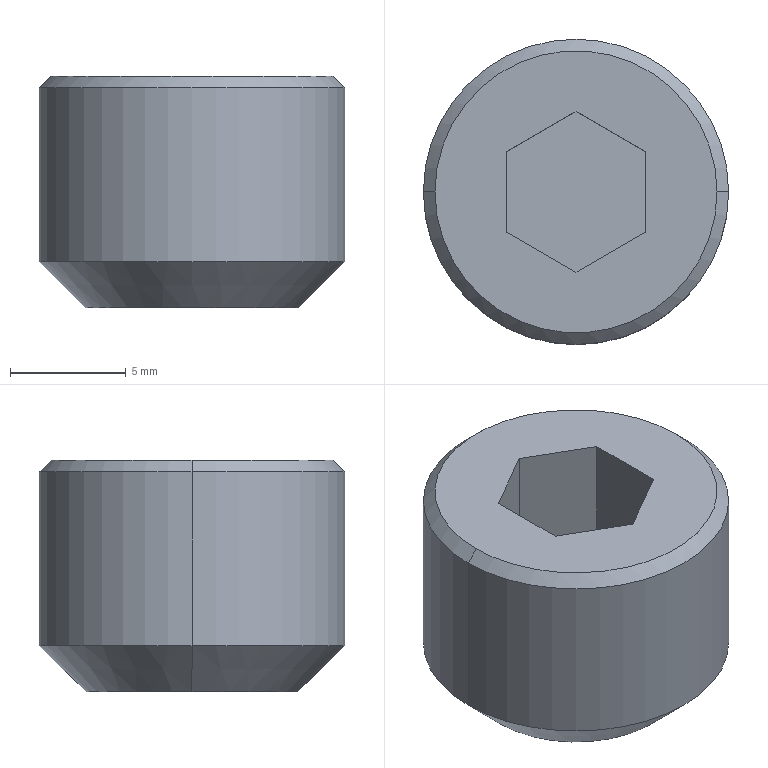Part | STEP file | 11-abp02-V2.0-V2.011 | 1 solid | 15 faces | box 13.16 x 13.16 x 10 mm | volume 1125 mm3 | plane 9 | cone 4 | cylinder 2 | commonest cylinder face diameters 13.16 x2
STEP:
#1=CARTESIAN_POINT('',(6.08,0.,10.));
#2=VERTEX_POINT('',#1);
#3=CARTESIAN_POINT('',(-6.08,0.,10.));
#4=VERTEX_POINT('',#3);
#5=CARTESIAN_POINT('',(0.,0.,10.));
#6=DIRECTION('',(0.,0.,1.));
#7=DIRECTION('',(1.,0.,0.));
#8=AXIS2_PLACEMENT_3D('',#5,#6,#7);
#9=CIRCLE('',#8,6.08);
#10=EDGE_CURVE('',#2,#4,#9,.T.);
#11=ORIENTED_EDGE('',*,*,#10,.F.);
#12=CARTESIAN_POINT('',(6.58,0.,9.5));
#13=VERTEX_POINT('',#12);
#14=CARTESIAN_POINT('',(6.08,0.,10.));
#15=DIRECTION('',(0.7071,0.,-0.7071));
#16=VECTOR('',#15,1000.);
#17=LINE('',#14,#16);
#18=EDGE_CURVE('',#2,#13,#17,.T.);
#19=ORIENTED_EDGE('',*,*,#18,.T.);
#20=CARTESIAN_POINT('',(-6.58,0.,9.5));
#21=VERTEX_POINT('',#20);
#22=CARTESIAN_POINT('',(0.,0.,9.5));
#23=DIRECTION('',(0.,0.,-1.));
#24=DIRECTION('',(1.,0.,0.));
#25=AXIS2_PLACEMENT_3D('',#22,#23,#24);
#26=CIRCLE('',#25,6.58);
#27=EDGE_CURVE('',#21,#13,#26,.T.);
#28=ORIENTED_EDGE('',*,*,#27,.F.);
#29=CARTESIAN_POINT('',(-6.08,0.,10.));
#30=DIRECTION('',(-0.7071,0.,-0.7071));
#31=VECTOR('',#30,1000.);
#32=LINE('',#29,#31);
#33=EDGE_CURVE('',#4,#21,#32,.T.);
#34=ORIENTED_EDGE('',*,*,#33,.F.);
#35=EDGE_LOOP('',(#11,#19,#28,#34));
#36=FACE_OUTER_BOUND('',#35,.T.);
#37=CARTESIAN_POINT('',(0.,0.,10.));
#38=DIRECTION('',(0.,0.,-1.));
#39=DIRECTION('',(-1.,0.,0.));
#40=AXIS2_PLACEMENT_3D('',#37,#38,#39);
#41=CONICAL_SURFACE('',#40,6.08,0.7854);
#42=ADVANCED_FACE('',(#36),#41,.T.);
#43=CARTESIAN_POINT('',(-4.58,0.,0.));
#44=VERTEX_POINT('',#43);
#45=CARTESIAN_POINT('',(4.58,0.,0.));
#46=VERTEX_POINT('',#45);
#47=CARTESIAN_POINT('',(0.,0.,0.));
#48=DIRECTION('',(0.,0.,-1.));
#49=DIRECTION('',(1.,0.,0.));
#50=AXIS2_PLACEMENT_3D('',#47,#48,#49);
#51=CIRCLE('',#50,4.58);
#52=EDGE_CURVE('',#44,#46,#51,.T.);
#53=ORIENTED_EDGE('',*,*,#52,.F.);
#54=CARTESIAN_POINT('',(-6.58,0.,2.));
#55=VERTEX_POINT('',#54);
#56=CARTESIAN_POINT('',(-6.58,0.,2.));
#57=DIRECTION('',(-0.7071,0.,0.7071));
#58=VECTOR('',#57,1000.);
#59=LINE('',#56,#58);
#60=EDGE_CURVE('',#44,#55,#59,.T.);
#61=ORIENTED_EDGE('',*,*,#60,.T.);
#62=CARTESIAN_POINT('',(6.58,0.,2.));
#63=VERTEX_POINT('',#62);
#64=CARTESIAN_POINT('',(0.,0.,2.));
#65=DIRECTION('',(0.,0.,1.));
#66=DIRECTION('',(1.,0.,0.));
#67=AXIS2_PLACEMENT_3D('',#64,#65,#66);
#68=CIRCLE('',#67,6.58);
#69=EDGE_CURVE('',#63,#55,#68,.T.);
#70=ORIENTED_EDGE('',*,*,#69,.F.);
#71=CARTESIAN_POINT('',(6.58,0.,2.));
#72=DIRECTION('',(0.7071,0.,0.7071));
#73=VECTOR('',#72,1000.);
#74=LINE('',#71,#73);
#75=EDGE_CURVE('',#46,#63,#74,.T.);
#76=ORIENTED_EDGE('',*,*,#75,.F.);
#77=EDGE_LOOP('',(#53,#61,#70,#76));
#78=FACE_OUTER_BOUND('',#77,.T.);
#79=CARTESIAN_POINT('',(0.,0.,2.));
#80=DIRECTION('',(0.,0.,1.));
#81=DIRECTION('',(1.,0.,0.));
#82=AXIS2_PLACEMENT_3D('',#79,#80,#81);
#83=CONICAL_SURFACE('',#82,6.58,0.7854);
#84=ADVANCED_FACE('',(#78),#83,.T.);
#85=ORIENTED_EDGE('',*,*,#27,.T.);
#86=CARTESIAN_POINT('',(6.58,0.,10.));
#87=DIRECTION('',(0.,0.,-1.));
#88=VECTOR('',#87,1000.);
#89=LINE('',#86,#88);
#90=EDGE_CURVE('',#13,#63,#89,.T.);
#91=ORIENTED_EDGE('',*,*,#90,.T.);
#92=ORIENTED_EDGE('',*,*,#69,.T.);
#93=CARTESIAN_POINT('',(-6.58,0.,10.));
#94=DIRECTION('',(0.,0.,-1.));
#95=VECTOR('',#94,1000.);
#96=LINE('',#93,#95);
#97=EDGE_CURVE('',#21,#55,#96,.T.);
#98=ORIENTED_EDGE('',*,*,#97,.F.);
#99=EDGE_LOOP('',(#85,#91,#92,#98));
#100=FACE_OUTER_BOUND('',#99,.T.);
#101=CARTESIAN_POINT('',(0.,0.,10.));
#102=DIRECTION('',(0.,0.,-1.));
#103=DIRECTION('',(-1.,0.,0.));
#104=AXIS2_PLACEMENT_3D('',#101,#102,#103);
#105=CYLINDRICAL_SURFACE('',#104,6.58);
#106=ADVANCED_FACE('',(#100),#105,.T.);
#107=ORIENTED_EDGE('',*,*,#90,.F.);
#108=CARTESIAN_POINT('',(0.,0.,9.5));
#109=DIRECTION('',(0.,0.,-1.));
#110=DIRECTION('',(1.,0.,0.));
#111=AXIS2_PLACEMENT_3D('',#108,#109,#110);
#112=CIRCLE('',#111,6.58);
#113=EDGE_CURVE('',#13,#21,#112,.T.);
#114=ORIENTED_EDGE('',*,*,#113,.T.);
#115=ORIENTED_EDGE('',*,*,#97,.T.);
#116=CARTESIAN_POINT('',(0.,0.,2.));
#117=DIRECTION('',(0.,0.,1.));
#118=DIRECTION('',(1.,0.,0.));
#119=AXIS2_PLACEMENT_3D('',#116,#117,#118);
#120=CIRCLE('',#119,6.58);
#121=EDGE_CURVE('',#55,#63,#120,.T.);
#122=ORIENTED_EDGE('',*,*,#121,.T.);
#123=EDGE_LOOP('',(#107,#114,#115,#122));
#124=FACE_OUTER_BOUND('',#123,.T.);
#125=CARTESIAN_POINT('',(0.,0.,10.));
#126=DIRECTION('',(0.,0.,-1.));
#127=DIRECTION('',(-1.,0.,0.));
#128=AXIS2_PLACEMENT_3D('',#125,#126,#127);
#129=CYLINDRICAL_SURFACE('',#128,6.58);
#130=ADVANCED_FACE('',(#124),#129,.T.);
#131=CARTESIAN_POINT('',(0.,0.,10.));
#132=DIRECTION('',(0.,0.,1.));
#133=DIRECTION('',(1.,0.,0.));
#134=AXIS2_PLACEMENT_3D('',#131,#132,#133);
#135=CIRCLE('',#134,6.08);
#136=EDGE_CURVE('',#4,#2,#135,.T.);
#137=ORIENTED_EDGE('',*,*,#136,.T.);
#138=ORIENTED_EDGE('',*,*,#10,.T.);
#139=EDGE_LOOP('',(#137,#138));
#140=FACE_OUTER_BOUND('',#139,.T.);
#141=CARTESIAN_POINT('',(3.,1.732,10.));
#142=VERTEX_POINT('',#141);
#143=CARTESIAN_POINT('',(0.,3.464,10.));
#144=VERTEX_POINT('',#143);
#145=CARTESIAN_POINT('',(3.,1.732,10.));
#146=DIRECTION('',(-0.866,0.5,0.));
#147=VECTOR('',#146,1000.);
#148=LINE('',#145,#147);
#149=EDGE_CURVE('',#142,#144,#148,.T.);
#150=ORIENTED_EDGE('',*,*,#149,.F.);
#151=CARTESIAN_POINT('',(3.,-1.732,10.));
#152=VERTEX_POINT('',#151);
#153=CARTESIAN_POINT('',(3.,-1.732,10.));
#154=DIRECTION('',(0.,1.,0.));
#155=VECTOR('',#154,1000.);
#156=LINE('',#153,#155);
#157=EDGE_CURVE('',#152,#142,#156,.T.);
#158=ORIENTED_EDGE('',*,*,#157,.F.);
#159=CARTESIAN_POINT('',(0.,-3.464,10.));
#160=VERTEX_POINT('',#159);
#161=CARTESIAN_POINT('',(0.,-3.464,10.));
#162=DIRECTION('',(0.866,0.5,0.));
#163=VECTOR('',#162,1000.);
#164=LINE('',#161,#163);
#165=EDGE_CURVE('',#160,#152,#164,.T.);
#166=ORIENTED_EDGE('',*,*,#165,.F.);
#167=CARTESIAN_POINT('',(-3.,-1.732,10.));
#168=VERTEX_POINT('',#167);
#169=CARTESIAN_POINT('',(-3.,-1.732,10.));
#170=DIRECTION('',(0.866,-0.5,0.));
#171=VECTOR('',#170,1000.);
#172=LINE('',#169,#171);
#173=EDGE_CURVE('',#168,#160,#172,.T.);
#174=ORIENTED_EDGE('',*,*,#173,.F.);
#175=CARTESIAN_POINT('',(-3.,1.732,10.));
#176=VERTEX_POINT('',#175);
#177=CARTESIAN_POINT('',(-3.,1.732,10.));
#178=DIRECTION('',(0.,-1.,0.));
#179=VECTOR('',#178,1000.);
#180=LINE('',#177,#179);
#181=EDGE_CURVE('',#176,#168,#180,.T.);
#182=ORIENTED_EDGE('',*,*,#181,.F.);
#183=CARTESIAN_POINT('',(0.,3.464,10.));
#184=DIRECTION('',(-0.866,-0.5,0.));
#185=VECTOR('',#184,1000.);
#186=LINE('',#183,#185);
#187=EDGE_CURVE('',#144,#176,#186,.T.);
#188=ORIENTED_EDGE('',*,*,#187,.F.);
#189=EDGE_LOOP('',(#150,#158,#166,#174,#182,#188));
#190=FACE_BOUND('',#189,.T.);
#191=CARTESIAN_POINT('',(0.,0.,10.));
#192=DIRECTION('',(0.,0.,1.));
#193=DIRECTION('',(1.,0.,0.));
#194=AXIS2_PLACEMENT_3D('',#191,#192,#193);
#195=PLANE('',#194);
#196=ADVANCED_FACE('',(#140,#190),#195,.T.);
#197=CARTESIAN_POINT('',(0.,0.,0.));
#198=DIRECTION('',(0.,0.,-1.));
#199=DIRECTION('',(1.,0.,0.));
#200=AXIS2_PLACEMENT_3D('',#197,#198,#199);
#201=CIRCLE('',#200,4.58);
#202=EDGE_CURVE('',#46,#44,#201,.T.);
#203=ORIENTED_EDGE('',*,*,#202,.T.);
#204=ORIENTED_EDGE('',*,*,#52,.T.);
#205=EDGE_LOOP('',(#203,#204));
#206=FACE_OUTER_BOUND('',#205,.T.);
#207=CARTESIAN_POINT('',(0.,0.,0.));
#208=DIRECTION('',(0.,0.,1.));
#209=DIRECTION('',(1.,0.,0.));
#210=AXIS2_PLACEMENT_3D('',#207,#208,#209);
#211=PLANE('',#210);
#212=ADVANCED_FACE('',(#206),#211,.F.);
#213=ORIENTED_EDGE('',*,*,#149,.T.);
#214=CARTESIAN_POINT('',(0.,3.464,5.));
#215=VERTEX_POINT('',#214);
#216=CARTESIAN_POINT('',(0.,3.464,5.));
#217=DIRECTION('',(0.,0.,1.));
#218=VECTOR('',#217,1000.);
#219=LINE('',#216,#218);
#220=EDGE_CURVE('',#215,#144,#219,.T.);
#221=ORIENTED_EDGE('',*,*,#220,.F.);
#222=CARTESIAN_POINT('',(3.,1.732,5.));
#223=VERTEX_POINT('',#222);
#224=CARTESIAN_POINT('',(3.,1.732,5.));
#225=DIRECTION('',(-0.866,0.5,0.));
#226=VECTOR('',#225,1000.);
#227=LINE('',#224,#226);
#228=EDGE_CURVE('',#223,#215,#227,.T.);
#229=ORIENTED_EDGE('',*,*,#228,.F.);
#230=CARTESIAN_POINT('',(3.,1.732,5.));
#231=DIRECTION('',(0.,0.,1.));
#232=VECTOR('',#231,1000.);
#233=LINE('',#230,#232);
#234=EDGE_CURVE('',#223,#142,#233,.T.);
#235=ORIENTED_EDGE('',*,*,#234,.T.);
#236=EDGE_LOOP('',(#213,#221,#229,#235));
#237=FACE_OUTER_BOUND('',#236,.T.);
#238=CARTESIAN_POINT('',(3.,1.732,5.));
#239=DIRECTION('',(0.5,0.866,0.));
#240=DIRECTION('',(-0.866,0.5,0.));
#241=AXIS2_PLACEMENT_3D('',#238,#239,#240);
#242=PLANE('',#241);
#243=ADVANCED_FACE('',(#237),#242,.F.);
#244=ORIENTED_EDGE('',*,*,#157,.T.);
#245=ORIENTED_EDGE('',*,*,#234,.F.);
#246=CARTESIAN_POINT('',(3.,-1.732,5.));
#247=VERTEX_POINT('',#246);
#248=CARTESIAN_POINT('',(3.,-1.732,5.));
#249=DIRECTION('',(0.,1.,0.));
#250=VECTOR('',#249,1000.);
#251=LINE('',#248,#250);
#252=EDGE_CURVE('',#247,#223,#251,.T.);
#253=ORIENTED_EDGE('',*,*,#252,.F.);
#254=CARTESIAN_POINT('',(3.,-1.732,5.));
#255=DIRECTION('',(0.,0.,1.));
#256=VECTOR('',#255,1000.);
#257=LINE('',#254,#256);
#258=EDGE_CURVE('',#247,#152,#257,.T.);
#259=ORIENTED_EDGE('',*,*,#258,.T.);
#260=EDGE_LOOP('',(#244,#245,#253,#259));
#261=FACE_OUTER_BOUND('',#260,.T.);
#262=CARTESIAN_POINT('',(3.,-1.732,5.));
#263=DIRECTION('',(1.,0.,0.));
#264=DIRECTION('',(0.,0.,-1.));
#265=AXIS2_PLACEMENT_3D('',#262,#263,#264);
#266=PLANE('',#265);
#267=ADVANCED_FACE('',(#261),#266,.F.);
#268=ORIENTED_EDGE('',*,*,#165,.T.);
#269=ORIENTED_EDGE('',*,*,#258,.F.);
#270=CARTESIAN_POINT('',(0.,-3.464,5.));
#271=VERTEX_POINT('',#270);
#272=CARTESIAN_POINT('',(0.,-3.464,5.));
#273=DIRECTION('',(0.866,0.5,0.));
#274=VECTOR('',#273,1000.);
#275=LINE('',#272,#274);
#276=EDGE_CURVE('',#271,#247,#275,.T.);
#277=ORIENTED_EDGE('',*,*,#276,.F.);
#278=CARTESIAN_POINT('',(0.,-3.464,5.));
#279=DIRECTION('',(0.,0.,1.));
#280=VECTOR('',#279,1000.);
#281=LINE('',#278,#280);
#282=EDGE_CURVE('',#271,#160,#281,.T.);
#283=ORIENTED_EDGE('',*,*,#282,.T.);
#284=EDGE_LOOP('',(#268,#269,#277,#283));
#285=FACE_OUTER_BOUND('',#284,.T.);
#286=CARTESIAN_POINT('',(0.,-3.464,5.));
#287=DIRECTION('',(0.5,-0.866,0.));
#288=DIRECTION('',(0.866,0.5,0.));
#289=AXIS2_PLACEMENT_3D('',#286,#287,#288);
#290=PLANE('',#289);
#291=ADVANCED_FACE('',(#285),#290,.F.);
#292=ORIENTED_EDGE('',*,*,#173,.T.);
#293=ORIENTED_EDGE('',*,*,#282,.F.);
#294=CARTESIAN_POINT('',(-3.,-1.732,5.));
#295=VERTEX_POINT('',#294);
#296=CARTESIAN_POINT('',(-3.,-1.732,5.));
#297=DIRECTION('',(0.866,-0.5,0.));
#298=VECTOR('',#297,1000.);
#299=LINE('',#296,#298);
#300=EDGE_CURVE('',#295,#271,#299,.T.);
#301=ORIENTED_EDGE('',*,*,#300,.F.);
#302=CARTESIAN_POINT('',(-3.,-1.732,5.));
#303=DIRECTION('',(0.,0.,1.));
#304=VECTOR('',#303,1000.);
#305=LINE('',#302,#304);
#306=EDGE_CURVE('',#295,#168,#305,.T.);
#307=ORIENTED_EDGE('',*,*,#306,.T.);
#308=EDGE_LOOP('',(#292,#293,#301,#307));
#309=FACE_OUTER_BOUND('',#308,.T.);
#310=CARTESIAN_POINT('',(-3.,-1.732,5.));
#311=DIRECTION('',(-0.5,-0.866,0.));
#312=DIRECTION('',(0.866,-0.5,0.));
#313=AXIS2_PLACEMENT_3D('',#310,#311,#312);
#314=PLANE('',#313);
#315=ADVANCED_FACE('',(#309),#314,.F.);
#316=ORIENTED_EDGE('',*,*,#181,.T.);
#317=ORIENTED_EDGE('',*,*,#306,.F.);
#318=CARTESIAN_POINT('',(-3.,1.732,5.));
#319=VERTEX_POINT('',#318);
#320=CARTESIAN_POINT('',(-3.,1.732,5.));
#321=DIRECTION('',(0.,-1.,0.));
#322=VECTOR('',#321,1000.);
#323=LINE('',#320,#322);
#324=EDGE_CURVE('',#319,#295,#323,.T.);
#325=ORIENTED_EDGE('',*,*,#324,.F.);
#326=CARTESIAN_POINT('',(-3.,1.732,5.));
#327=DIRECTION('',(0.,0.,1.));
#328=VECTOR('',#327,1000.);
#329=LINE('',#326,#328);
#330=EDGE_CURVE('',#319,#176,#329,.T.);
#331=ORIENTED_EDGE('',*,*,#330,.T.);
#332=EDGE_LOOP('',(#316,#317,#325,#331));
#333=FACE_OUTER_BOUND('',#332,.T.);
#334=CARTESIAN_POINT('',(-3.,1.732,5.));
#335=DIRECTION('',(-1.,0.,0.));
#336=DIRECTION('',(0.,0.,1.));
#337=AXIS2_PLACEMENT_3D('',#334,#335,#336);
#338=PLANE('',#337);
#339=ADVANCED_FACE('',(#333),#338,.F.);
#340=ORIENTED_EDGE('',*,*,#187,.T.);
#341=ORIENTED_EDGE('',*,*,#330,.F.);
#342=CARTESIAN_POINT('',(0.,3.464,5.));
#343=DIRECTION('',(-0.866,-0.5,0.));
#344=VECTOR('',#343,1000.);
#345=LINE('',#342,#344);
#346=EDGE_CURVE('',#215,#319,#345,.T.);
#347=ORIENTED_EDGE('',*,*,#346,.F.);
#348=ORIENTED_EDGE('',*,*,#220,.T.);
#349=EDGE_LOOP('',(#340,#341,#347,#348));
#350=FACE_OUTER_BOUND('',#349,.T.);
#351=CARTESIAN_POINT('',(0.,3.464,5.));
#352=DIRECTION('',(-0.5,0.866,0.));
#353=DIRECTION('',(-0.866,-0.5,0.));
#354=AXIS2_PLACEMENT_3D('',#351,#352,#353);
#355=PLANE('',#354);
#356=ADVANCED_FACE('',(#350),#355,.F.);
#357=ORIENTED_EDGE('',*,*,#228,.T.);
#358=ORIENTED_EDGE('',*,*,#346,.T.);
#359=ORIENTED_EDGE('',*,*,#324,.T.);
#360=ORIENTED_EDGE('',*,*,#300,.T.);
#361=ORIENTED_EDGE('',*,*,#276,.T.);
#362=ORIENTED_EDGE('',*,*,#252,.T.);
#363=EDGE_LOOP('',(#357,#358,#359,#360,#361,#362));
#364=FACE_OUTER_BOUND('',#363,.T.);
#365=CARTESIAN_POINT('',(0.,0.,5.));
#366=DIRECTION('',(0.,0.,1.));
#367=DIRECTION('',(1.,0.,0.));
#368=AXIS2_PLACEMENT_3D('',#365,#366,#367);
#369=PLANE('',#368);
#370=ADVANCED_FACE('',(#364),#369,.T.);
#371=ORIENTED_EDGE('',*,*,#60,.F.);
#372=ORIENTED_EDGE('',*,*,#202,.F.);
#373=ORIENTED_EDGE('',*,*,#75,.T.);
#374=ORIENTED_EDGE('',*,*,#121,.F.);
#375=EDGE_LOOP('',(#371,#372,#373,#374));
#376=FACE_OUTER_BOUND('',#375,.T.);
#377=CARTESIAN_POINT('',(0.,0.,2.));
#378=DIRECTION('',(0.,0.,1.));
#379=DIRECTION('',(1.,0.,0.));
#380=AXIS2_PLACEMENT_3D('',#377,#378,#379);
#381=CONICAL_SURFACE('',#380,6.58,0.7854);
#382=ADVANCED_FACE('',(#376),#381,.T.);
#383=ORIENTED_EDGE('',*,*,#18,.F.);
#384=ORIENTED_EDGE('',*,*,#136,.F.);
#385=ORIENTED_EDGE('',*,*,#33,.T.);
#386=ORIENTED_EDGE('',*,*,#113,.F.);
#387=EDGE_LOOP('',(#383,#384,#385,#386));
#388=FACE_OUTER_BOUND('',#387,.T.);
#389=CARTESIAN_POINT('',(0.,0.,10.));
#390=DIRECTION('',(0.,0.,-1.));
#391=DIRECTION('',(-1.,0.,0.));
#392=AXIS2_PLACEMENT_3D('',#389,#390,#391);
#393=CONICAL_SURFACE('',#392,6.08,0.7854);
#394=ADVANCED_FACE('',(#388),#393,.T.);
#395=CLOSED_SHELL('',(#42,#84,#106,#130,#196,#212,#243,#267,#291,#315,#339,#356,#370,#382,#394));
#396=MANIFOLD_SOLID_BREP('',#395);
#397=CARTESIAN_POINT('',(0.,0.,0.));
#398=DIRECTION('',(0.,0.,1.));
#399=DIRECTION('',(1.,0.,0.));
#400=AXIS2_PLACEMENT_3D('',#397,#398,#399);
#401=(LENGTH_UNIT()NAMED_UNIT(*)SI_UNIT(.MILLI.,.METRE.));
#402=UNCERTAINTY_MEASURE_WITH_UNIT(LENGTH_MEASURE(0.00001),#401,'','');
#403=(NAMED_UNIT(*)PLANE_ANGLE_UNIT()SI_UNIT($,.RADIAN.));
#404=(NAMED_UNIT(*)SI_UNIT($,.STERADIAN.)SOLID_ANGLE_UNIT());
#405=(GEOMETRIC_REPRESENTATION_CONTEXT(3)GLOBAL_UNCERTAINTY_ASSIGNED_CONTEXT((#402))GLOBAL_UNIT_ASSIGNED_CONTEXT((#401,#403,#404))REPRESENTATION_CONTEXT('',''));
#406=ADVANCED_BREP_SHAPE_REPRESENTATION('',(#396,#400),#405);